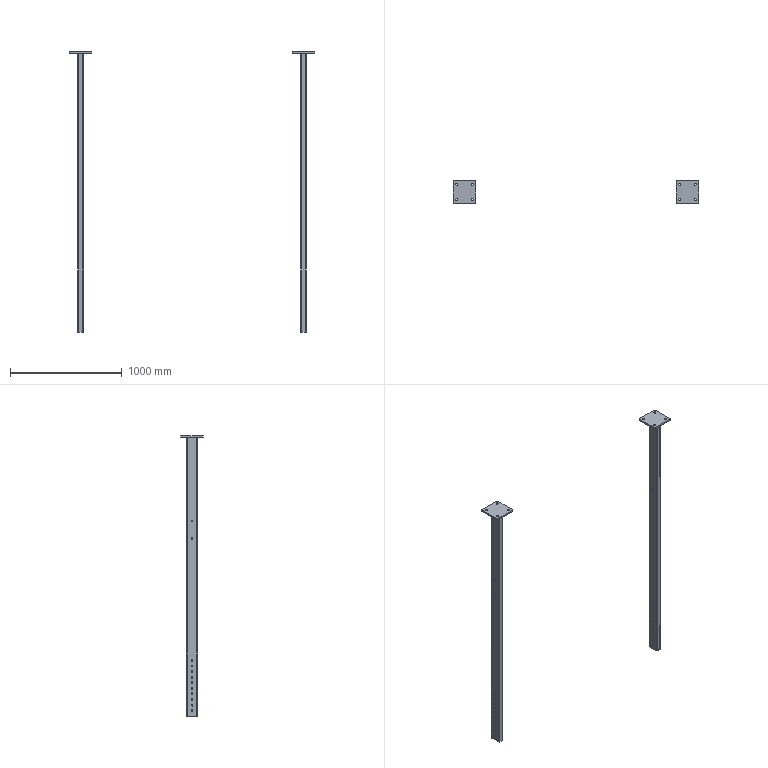Part | SolidWorks | features HoleWzd 4, Fillet 2, ICE 2, MirrorSolid 2, 3DProfileFeature 1, LPattern 1, WeldMemberFeat 1, WeldmentFeature 1 | 4 solids | 168 faces | box 2200 x 200 x 2514 mm | volume 6513642 mm3 | cylinder 136 | plane 32 | commonest cylinder face diameters 17.5 x96 19 x16 8 x8 16 x8 20 x8